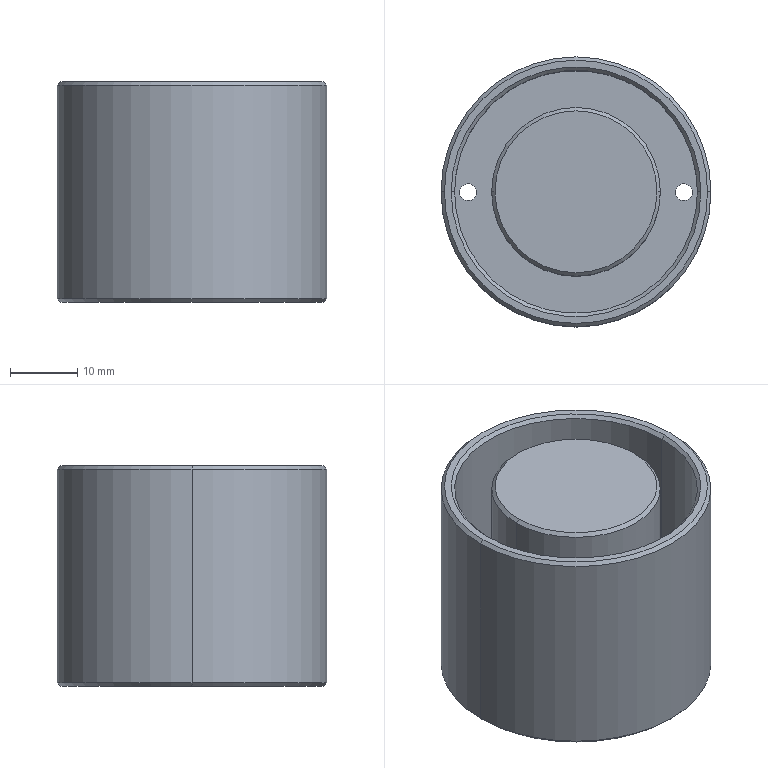Part | STEP file | 1 solid | 28 faces | box 40 x 40 x 32.7 mm | volume 26304 mm3 | cylinder 14 | cone 8 | plane 6 | commonest cylinder face diameters 2.5 x4 3.3 x4 25 x2 36 x2 40 x2